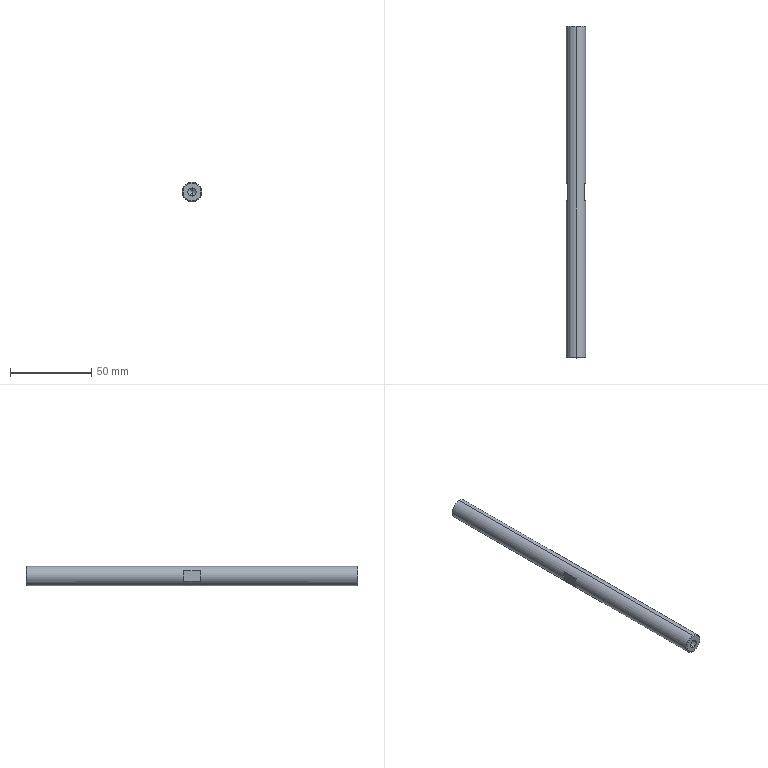Part | STEP file | 0-19-13 Support rod | 1 solid | 22 faces | box 12 x 204 x 12 mm | volume 22364 mm3 | cone 8 | plane 8 | cylinder 6 | commonest cylinder face diameters 5 x4 12 x2
STEP:
#1=CARTESIAN_POINT('',(0.,0.,0.));
#2=DIRECTION('',(0.,0.,1.));
#3=DIRECTION('',(1.,0.,0.));
#4=AXIS2_PLACEMENT_3D('',#1,#2,#3);
#5=CARTESIAN_POINT('',(0.,102.,5.5));
#6=VERTEX_POINT('',#5);
#7=CARTESIAN_POINT('',(0.,102.,-5.5));
#8=VERTEX_POINT('',#7);
#9=CARTESIAN_POINT('',(0.,102.,0.));
#10=DIRECTION('',(0.,1.,0.));
#11=DIRECTION('',(0.,0.,1.));
#12=AXIS2_PLACEMENT_3D('',#9,#10,#11);
#13=CIRCLE('',#12,5.5);
#14=CARTESIAN_POINT('',(0.,101.5,0.));
#15=DIRECTION('',(0.,-1.,0.));
#16=DIRECTION('',(0.,0.,-1.));
#17=AXIS2_PLACEMENT_3D('',#14,#15,#16);
#18=CONICAL_SURFACE('',#17,6.,0.7854);
#19=CARTESIAN_POINT('',(3.142,-0.5));
#20=DIRECTION('',(-1.,0.));
#21=VECTOR('',#20,1.);
#22=LINE('',#19,#21);
#23=(GEOMETRIC_REPRESENTATION_CONTEXT(2)PARAMETRIC_REPRESENTATION_CONTEXT()REPRESENTATION_CONTEXT('',''));
#24=DEFINITIONAL_REPRESENTATION('',(#22),#23);
#25=PCURVE('',#18,#24);
#26=CARTESIAN_POINT('',(6.,102.,0.));
#27=DIRECTION('',(0.,1.,0.));
#28=DIRECTION('',(0.,0.,1.));
#29=AXIS2_PLACEMENT_3D('',#26,#27,#28);
#30=PLANE('',#29);
#31=CARTESIAN_POINT('',(0.,-6.));
#32=DIRECTION('',(1.,0.));
#33=AXIS2_PLACEMENT_2D('',#31,#32);
#34=CIRCLE('',#33,5.5);
#35=(GEOMETRIC_REPRESENTATION_CONTEXT(2)PARAMETRIC_REPRESENTATION_CONTEXT()REPRESENTATION_CONTEXT('',''));
#36=DEFINITIONAL_REPRESENTATION('',(#34),#35);
#37=PCURVE('',#30,#36);
#38=SURFACE_CURVE('',#13,(#25,#37),.PCURVE_S1.);
#39=EDGE_CURVE('',#6,#8,#38,.T.);
#40=ORIENTED_EDGE('',*,*,#39,.F.);
#41=CARTESIAN_POINT('',(0.,101.5,6.));
#42=VERTEX_POINT('',#41);
#43=CARTESIAN_POINT('',(0.,101.5,6.));
#44=DIRECTION('',(0.,-0.7071,0.7071));
#45=VECTOR('',#44,1.);
#46=LINE('',#43,#45);
#47=CARTESIAN_POINT('',(3.142,0.));
#48=DIRECTION('',(0.,1.));
#49=VECTOR('',#48,1.);
#50=LINE('',#47,#49);
#51=(GEOMETRIC_REPRESENTATION_CONTEXT(2)PARAMETRIC_REPRESENTATION_CONTEXT()REPRESENTATION_CONTEXT('',''));
#52=DEFINITIONAL_REPRESENTATION('',(#50),#51);
#53=PCURVE('',#18,#52);
#54=CARTESIAN_POINT('',(0.,101.5,0.));
#55=DIRECTION('',(0.,-1.,0.));
#56=DIRECTION('',(0.,0.,-1.));
#57=AXIS2_PLACEMENT_3D('',#54,#55,#56);
#58=CONICAL_SURFACE('',#57,6.,0.7854);
#59=CARTESIAN_POINT('',(3.142,0.));
#60=DIRECTION('',(0.,1.));
#61=VECTOR('',#60,1.);
#62=LINE('',#59,#61);
#63=(GEOMETRIC_REPRESENTATION_CONTEXT(2)PARAMETRIC_REPRESENTATION_CONTEXT()REPRESENTATION_CONTEXT('',''));
#64=DEFINITIONAL_REPRESENTATION('',(#62),#63);
#65=PCURVE('',#58,#64);
#66=SURFACE_CURVE('',#46,(#53,#65),.PCURVE_S1.);
#67=EDGE_CURVE('',#6,#42,#66,.T.);
#68=ORIENTED_EDGE('',*,*,#67,.T.);
#69=CARTESIAN_POINT('',(0.,101.5,-6.));
#70=VERTEX_POINT('',#69);
#71=CARTESIAN_POINT('',(0.,101.5,0.));
#72=DIRECTION('',(0.,-1.,0.));
#73=DIRECTION('',(0.,0.,1.));
#74=AXIS2_PLACEMENT_3D('',#71,#72,#73);
#75=CIRCLE('',#74,6.);
#76=CARTESIAN_POINT('',(-3.142,0.));
#77=DIRECTION('',(1.,0.));
#78=VECTOR('',#77,1.);
#79=LINE('',#76,#78);
#80=(GEOMETRIC_REPRESENTATION_CONTEXT(2)PARAMETRIC_REPRESENTATION_CONTEXT()REPRESENTATION_CONTEXT('',''));
#81=DEFINITIONAL_REPRESENTATION('',(#79),#80);
#82=PCURVE('',#18,#81);
#83=CARTESIAN_POINT('',(0.,0.,0.));
#84=DIRECTION('',(0.,-1.,0.));
#85=DIRECTION('',(0.,0.,-1.));
#86=AXIS2_PLACEMENT_3D('',#83,#84,#85);
#87=CYLINDRICAL_SURFACE('',#86,6.);
#88=CARTESIAN_POINT('',(-3.142,-101.5));
#89=DIRECTION('',(1.,0.));
#90=VECTOR('',#89,1.);
#91=LINE('',#88,#90);
#92=(GEOMETRIC_REPRESENTATION_CONTEXT(2)PARAMETRIC_REPRESENTATION_CONTEXT()REPRESENTATION_CONTEXT('',''));
#93=DEFINITIONAL_REPRESENTATION('',(#91),#92);
#94=PCURVE('',#87,#93);
#95=SURFACE_CURVE('',#75,(#82,#94),.PCURVE_S1.);
#96=EDGE_CURVE('',#70,#42,#95,.T.);
#97=ORIENTED_EDGE('',*,*,#96,.F.);
#98=CARTESIAN_POINT('',(0.,101.5,-6.));
#99=DIRECTION('',(0.,-0.7071,-0.7071));
#100=VECTOR('',#99,1.);
#101=LINE('',#98,#100);
#102=CARTESIAN_POINT('',(0.,0.));
#103=DIRECTION('',(0.,1.));
#104=VECTOR('',#103,1.);
#105=LINE('',#102,#104);
#106=(GEOMETRIC_REPRESENTATION_CONTEXT(2)PARAMETRIC_REPRESENTATION_CONTEXT()REPRESENTATION_CONTEXT('',''));
#107=DEFINITIONAL_REPRESENTATION('',(#105),#106);
#108=PCURVE('',#18,#107);
#109=CARTESIAN_POINT('',(6.283,0.));
#110=DIRECTION('',(0.,1.));
#111=VECTOR('',#110,1.);
#112=LINE('',#109,#111);
#113=(GEOMETRIC_REPRESENTATION_CONTEXT(2)PARAMETRIC_REPRESENTATION_CONTEXT()REPRESENTATION_CONTEXT('',''));
#114=DEFINITIONAL_REPRESENTATION('',(#112),#113);
#115=PCURVE('',#58,#114);
#116=SURFACE_CURVE('',#101,(#108,#115),.PCURVE_S1.);
#117=EDGE_CURVE('',#8,#70,#116,.T.);
#118=ORIENTED_EDGE('',*,*,#117,.F.);
#119=EDGE_LOOP('',(#40,#68,#97,#118));
#120=FACE_BOUND('',#119,.T.);
#121=ADVANCED_FACE('',(#120),#18,.T.);
#122=CARTESIAN_POINT('',(0.,-102.,-5.5));
#123=VERTEX_POINT('',#122);
#124=CARTESIAN_POINT('',(0.,-102.,5.5));
#125=VERTEX_POINT('',#124);
#126=CARTESIAN_POINT('',(0.,-102.,0.));
#127=DIRECTION('',(0.,-1.,0.));
#128=DIRECTION('',(0.,0.,-1.));
#129=AXIS2_PLACEMENT_3D('',#126,#127,#128);
#130=CIRCLE('',#129,5.5);
#131=CARTESIAN_POINT('',(0.,-102.,0.));
#132=DIRECTION('',(0.,1.,0.));
#133=DIRECTION('',(0.,0.,1.));
#134=AXIS2_PLACEMENT_3D('',#131,#132,#133);
#135=CONICAL_SURFACE('',#134,5.5,0.7854);
#136=CARTESIAN_POINT('',(3.142,0.));
#137=DIRECTION('',(-1.,0.));
#138=VECTOR('',#137,1.);
#139=LINE('',#136,#138);
#140=(GEOMETRIC_REPRESENTATION_CONTEXT(2)PARAMETRIC_REPRESENTATION_CONTEXT()REPRESENTATION_CONTEXT('',''));
#141=DEFINITIONAL_REPRESENTATION('',(#139),#140);
#142=PCURVE('',#135,#141);
#143=CARTESIAN_POINT('',(6.,-102.,0.));
#144=DIRECTION('',(0.,-1.,0.));
#145=DIRECTION('',(0.,0.,-1.));
#146=AXIS2_PLACEMENT_3D('',#143,#144,#145);
#147=PLANE('',#146);
#148=CARTESIAN_POINT('',(0.,-6.));
#149=DIRECTION('',(1.,0.));
#150=AXIS2_PLACEMENT_2D('',#148,#149);
#151=CIRCLE('',#150,5.5);
#152=(GEOMETRIC_REPRESENTATION_CONTEXT(2)PARAMETRIC_REPRESENTATION_CONTEXT()REPRESENTATION_CONTEXT('',''));
#153=DEFINITIONAL_REPRESENTATION('',(#151),#152);
#154=PCURVE('',#147,#153);
#155=SURFACE_CURVE('',#130,(#142,#154),.PCURVE_S1.);
#156=EDGE_CURVE('',#123,#125,#155,.T.);
#157=ORIENTED_EDGE('',*,*,#156,.F.);
#158=CARTESIAN_POINT('',(0.,-101.5,-6.));
#159=VERTEX_POINT('',#158);
#160=CARTESIAN_POINT('',(0.,-102.,-5.5));
#161=DIRECTION('',(0.,0.7071,-0.7071));
#162=VECTOR('',#161,1.);
#163=LINE('',#160,#162);
#164=CARTESIAN_POINT('',(3.142,0.));
#165=DIRECTION('',(0.,1.));
#166=VECTOR('',#165,1.);
#167=LINE('',#164,#166);
#168=(GEOMETRIC_REPRESENTATION_CONTEXT(2)PARAMETRIC_REPRESENTATION_CONTEXT()REPRESENTATION_CONTEXT('',''));
#169=DEFINITIONAL_REPRESENTATION('',(#167),#168);
#170=PCURVE('',#135,#169);
#171=CARTESIAN_POINT('',(0.,-102.,0.));
#172=DIRECTION('',(0.,1.,0.));
#173=DIRECTION('',(0.,0.,1.));
#174=AXIS2_PLACEMENT_3D('',#171,#172,#173);
#175=CONICAL_SURFACE('',#174,5.5,0.7854);
#176=CARTESIAN_POINT('',(3.142,0.));
#177=DIRECTION('',(0.,1.));
#178=VECTOR('',#177,1.);
#179=LINE('',#176,#178);
#180=(GEOMETRIC_REPRESENTATION_CONTEXT(2)PARAMETRIC_REPRESENTATION_CONTEXT()REPRESENTATION_CONTEXT('',''));
#181=DEFINITIONAL_REPRESENTATION('',(#179),#180);
#182=PCURVE('',#175,#181);
#183=SURFACE_CURVE('',#163,(#170,#182),.PCURVE_S1.);
#184=EDGE_CURVE('',#123,#159,#183,.T.);
#185=ORIENTED_EDGE('',*,*,#184,.T.);
#186=CARTESIAN_POINT('',(0.,-101.5,6.));
#187=VERTEX_POINT('',#186);
#188=CARTESIAN_POINT('',(0.,-101.5,0.));
#189=DIRECTION('',(0.,1.,0.));
#190=DIRECTION('',(0.,0.,-1.));
#191=AXIS2_PLACEMENT_3D('',#188,#189,#190);
#192=CIRCLE('',#191,6.);
#193=CARTESIAN_POINT('',(-3.142,0.5));
#194=DIRECTION('',(1.,0.));
#195=VECTOR('',#194,1.);
#196=LINE('',#193,#195);
#197=(GEOMETRIC_REPRESENTATION_CONTEXT(2)PARAMETRIC_REPRESENTATION_CONTEXT()REPRESENTATION_CONTEXT('',''));
#198=DEFINITIONAL_REPRESENTATION('',(#196),#197);
#199=PCURVE('',#135,#198);
#200=CARTESIAN_POINT('',(6.283,101.5));
#201=DIRECTION('',(-1.,0.));
#202=VECTOR('',#201,1.);
#203=LINE('',#200,#202);
#204=(GEOMETRIC_REPRESENTATION_CONTEXT(2)PARAMETRIC_REPRESENTATION_CONTEXT()REPRESENTATION_CONTEXT('',''));
#205=DEFINITIONAL_REPRESENTATION('',(#203),#204);
#206=PCURVE('',#87,#205);
#207=SURFACE_CURVE('',#192,(#199,#206),.PCURVE_S1.);
#208=EDGE_CURVE('',#187,#159,#207,.T.);
#209=ORIENTED_EDGE('',*,*,#208,.F.);
#210=CARTESIAN_POINT('',(0.,-102.,5.5));
#211=DIRECTION('',(0.,0.7071,0.7071));
#212=VECTOR('',#211,1.);
#213=LINE('',#210,#212);
#214=CARTESIAN_POINT('',(0.,0.));
#215=DIRECTION('',(0.,1.));
#216=VECTOR('',#215,1.);
#217=LINE('',#214,#216);
#218=(GEOMETRIC_REPRESENTATION_CONTEXT(2)PARAMETRIC_REPRESENTATION_CONTEXT()REPRESENTATION_CONTEXT('',''));
#219=DEFINITIONAL_REPRESENTATION('',(#217),#218);
#220=PCURVE('',#135,#219);
#221=CARTESIAN_POINT('',(6.283,0.));
#222=DIRECTION('',(0.,1.));
#223=VECTOR('',#222,1.);
#224=LINE('',#221,#223);
#225=(GEOMETRIC_REPRESENTATION_CONTEXT(2)PARAMETRIC_REPRESENTATION_CONTEXT()REPRESENTATION_CONTEXT('',''));
#226=DEFINITIONAL_REPRESENTATION('',(#224),#225);
#227=PCURVE('',#175,#226);
#228=SURFACE_CURVE('',#213,(#220,#227),.PCURVE_S1.);
#229=EDGE_CURVE('',#125,#187,#228,.T.);
#230=ORIENTED_EDGE('',*,*,#229,.F.);
#231=EDGE_LOOP('',(#157,#185,#209,#230));
#232=FACE_BOUND('',#231,.T.);
#233=ADVANCED_FACE('',(#232),#135,.T.);
#234=CARTESIAN_POINT('',(0.,-87.,-2.5));
#235=VERTEX_POINT('',#234);
#236=CARTESIAN_POINT('',(0.,-102.,-2.5));
#237=VERTEX_POINT('',#236);
#238=CARTESIAN_POINT('',(0.,-102.,-2.5));
#239=DIRECTION('',(0.,-1.,0.));
#240=VECTOR('',#239,1.);
#241=LINE('',#238,#240);
#242=CARTESIAN_POINT('',(0.,-102.,0.));
#243=DIRECTION('',(0.,-1.,0.));
#244=DIRECTION('',(0.,0.,-1.));
#245=AXIS2_PLACEMENT_3D('',#242,#243,#244);
#246=CYLINDRICAL_SURFACE('',#245,2.5);
#247=CARTESIAN_POINT('',(6.283,0.));
#248=DIRECTION('',(0.,1.));
#249=VECTOR('',#248,1.);
#250=LINE('',#247,#249);
#251=(GEOMETRIC_REPRESENTATION_CONTEXT(2)PARAMETRIC_REPRESENTATION_CONTEXT()REPRESENTATION_CONTEXT('',''));
#252=DEFINITIONAL_REPRESENTATION('',(#250),#251);
#253=PCURVE('',#246,#252);
#254=CARTESIAN_POINT('',(0.,-102.,0.));
#255=DIRECTION('',(0.,-1.,0.));
#256=DIRECTION('',(0.,0.,-1.));
#257=AXIS2_PLACEMENT_3D('',#254,#255,#256);
#258=CYLINDRICAL_SURFACE('',#257,2.5);
#259=CARTESIAN_POINT('',(0.,0.));
#260=DIRECTION('',(0.,1.));
#261=VECTOR('',#260,1.);
#262=LINE('',#259,#261);
#263=(GEOMETRIC_REPRESENTATION_CONTEXT(2)PARAMETRIC_REPRESENTATION_CONTEXT()REPRESENTATION_CONTEXT('',''));
#264=DEFINITIONAL_REPRESENTATION('',(#262),#263);
#265=PCURVE('',#258,#264);
#266=SURFACE_CURVE('',#241,(#253,#265),.PCURVE_S1.);
#267=EDGE_CURVE('',#235,#237,#266,.T.);
#268=ORIENTED_EDGE('',*,*,#267,.T.);
#269=CARTESIAN_POINT('',(0.,-102.,2.5));
#270=VERTEX_POINT('',#269);
#271=CARTESIAN_POINT('',(0.,-102.,0.));
#272=DIRECTION('',(0.,-1.,0.));
#273=DIRECTION('',(0.,0.,-1.));
#274=AXIS2_PLACEMENT_3D('',#271,#272,#273);
#275=CIRCLE('',#274,2.5);
#276=CARTESIAN_POINT('',(0.,0.));
#277=DIRECTION('',(1.,0.));
#278=VECTOR('',#277,1.);
#279=LINE('',#276,#278);
#280=(GEOMETRIC_REPRESENTATION_CONTEXT(2)PARAMETRIC_REPRESENTATION_CONTEXT()REPRESENTATION_CONTEXT('',''));
#281=DEFINITIONAL_REPRESENTATION('',(#279),#280);
#282=PCURVE('',#246,#281);
#283=CARTESIAN_POINT('',(0.,-6.));
#284=DIRECTION('',(1.,0.));
#285=AXIS2_PLACEMENT_2D('',#283,#284);
#286=CIRCLE('',#285,2.5);
#287=(GEOMETRIC_REPRESENTATION_CONTEXT(2)PARAMETRIC_REPRESENTATION_CONTEXT()REPRESENTATION_CONTEXT('',''));
#288=DEFINITIONAL_REPRESENTATION('',(#286),#287);
#289=PCURVE('',#147,#288);
#290=SURFACE_CURVE('',#275,(#282,#289),.PCURVE_S1.);
#291=EDGE_CURVE('',#270,#237,#290,.T.);
#292=ORIENTED_EDGE('',*,*,#291,.F.);
#293=CARTESIAN_POINT('',(0.,-87.,2.5));
#294=VERTEX_POINT('',#293);
#295=CARTESIAN_POINT('',(0.,-102.,2.5));
#296=DIRECTION('',(0.,-1.,0.));
#297=VECTOR('',#296,1.);
#298=LINE('',#295,#297);
#299=CARTESIAN_POINT('',(3.142,0.));
#300=DIRECTION('',(0.,1.));
#301=VECTOR('',#300,1.);
#302=LINE('',#299,#301);
#303=(GEOMETRIC_REPRESENTATION_CONTEXT(2)PARAMETRIC_REPRESENTATION_CONTEXT()REPRESENTATION_CONTEXT('',''));
#304=DEFINITIONAL_REPRESENTATION('',(#302),#303);
#305=PCURVE('',#246,#304);
#306=CARTESIAN_POINT('',(3.142,0.));
#307=DIRECTION('',(0.,1.));
#308=VECTOR('',#307,1.);
#309=LINE('',#306,#308);
#310=(GEOMETRIC_REPRESENTATION_CONTEXT(2)PARAMETRIC_REPRESENTATION_CONTEXT()REPRESENTATION_CONTEXT('',''));
#311=DEFINITIONAL_REPRESENTATION('',(#309),#310);
#312=PCURVE('',#258,#311);
#313=SURFACE_CURVE('',#298,(#305,#312),.PCURVE_S1.);
#314=EDGE_CURVE('',#294,#270,#313,.T.);
#315=ORIENTED_EDGE('',*,*,#314,.F.);
#316=CARTESIAN_POINT('',(0.,-87.,0.));
#317=DIRECTION('',(0.,-1.,0.));
#318=DIRECTION('',(0.,0.,-1.));
#319=AXIS2_PLACEMENT_3D('',#316,#317,#318);
#320=CIRCLE('',#319,2.5);
#321=CARTESIAN_POINT('',(0.,-15.));
#322=DIRECTION('',(1.,0.));
#323=VECTOR('',#322,1.);
#324=LINE('',#321,#323);
#325=(GEOMETRIC_REPRESENTATION_CONTEXT(2)PARAMETRIC_REPRESENTATION_CONTEXT()REPRESENTATION_CONTEXT('',''));
#326=DEFINITIONAL_REPRESENTATION('',(#324),#325);
#327=PCURVE('',#246,#326);
#328=CARTESIAN_POINT('',(0.,-87.,0.));
#329=DIRECTION('',(0.,-1.,0.));
#330=DIRECTION('',(0.,0.,-1.));
#331=AXIS2_PLACEMENT_3D('',#328,#329,#330);
#332=CONICAL_SURFACE('',#331,2.5,1.03);
#333=CARTESIAN_POINT('',(0.,0.));
#334=DIRECTION('',(1.,0.));
#335=VECTOR('',#334,1.);
#336=LINE('',#333,#335);
#337=(GEOMETRIC_REPRESENTATION_CONTEXT(2)PARAMETRIC_REPRESENTATION_CONTEXT()REPRESENTATION_CONTEXT('',''));
#338=DEFINITIONAL_REPRESENTATION('',(#336),#337);
#339=PCURVE('',#332,#338);
#340=SURFACE_CURVE('',#320,(#327,#339),.PCURVE_S1.);
#341=EDGE_CURVE('',#294,#235,#340,.T.);
#342=ORIENTED_EDGE('',*,*,#341,.T.);
#343=EDGE_LOOP('',(#268,#292,#315,#342));
#344=FACE_BOUND('',#343,.F.);
#345=ADVANCED_FACE('',(#344),#246,.F.);
#346=ORIENTED_EDGE('',*,*,#341,.F.);
#347=CARTESIAN_POINT('',(0.,-85.498,0.));
#348=VERTEX_POINT('',#347);
#349=CARTESIAN_POINT('',(0.,-87.,2.5));
#350=DIRECTION('',(0.,-0.515,0.8572));
#351=VECTOR('',#350,1.);
#352=LINE('',#349,#351);
#353=CARTESIAN_POINT('',(3.142,0.));
#354=DIRECTION('',(0.,1.));
#355=VECTOR('',#354,1.);
#356=LINE('',#353,#355);
#357=(GEOMETRIC_REPRESENTATION_CONTEXT(2)PARAMETRIC_REPRESENTATION_CONTEXT()REPRESENTATION_CONTEXT('',''));
#358=DEFINITIONAL_REPRESENTATION('',(#356),#357);
#359=PCURVE('',#332,#358);
#360=CARTESIAN_POINT('',(0.,-87.,0.));
#361=DIRECTION('',(0.,-1.,0.));
#362=DIRECTION('',(0.,0.,-1.));
#363=AXIS2_PLACEMENT_3D('',#360,#361,#362);
#364=CONICAL_SURFACE('',#363,2.5,1.03);
#365=CARTESIAN_POINT('',(3.142,0.));
#366=DIRECTION('',(0.,1.));
#367=VECTOR('',#366,1.);
#368=LINE('',#365,#367);
#369=(GEOMETRIC_REPRESENTATION_CONTEXT(2)PARAMETRIC_REPRESENTATION_CONTEXT()REPRESENTATION_CONTEXT('',''));
#370=DEFINITIONAL_REPRESENTATION('',(#368),#369);
#371=PCURVE('',#364,#370);
#372=SURFACE_CURVE('',#352,(#359,#371),.PCURVE_S1.);
#373=EDGE_CURVE('',#348,#294,#372,.T.);
#374=ORIENTED_EDGE('',*,*,#373,.F.);
#375=CARTESIAN_POINT('',(0.,-87.,-2.5));
#376=DIRECTION('',(0.,-0.515,-0.8572));
#377=VECTOR('',#376,1.);
#378=LINE('',#375,#377);
#379=CARTESIAN_POINT('',(6.283,0.));
#380=DIRECTION('',(0.,1.));
#381=VECTOR('',#380,1.);
#382=LINE('',#379,#381);
#383=(GEOMETRIC_REPRESENTATION_CONTEXT(2)PARAMETRIC_REPRESENTATION_CONTEXT()REPRESENTATION_CONTEXT('',''));
#384=DEFINITIONAL_REPRESENTATION('',(#382),#383);
#385=PCURVE('',#332,#384);
#386=CARTESIAN_POINT('',(0.,0.));
#387=DIRECTION('',(0.,1.));
#388=VECTOR('',#387,1.);
#389=LINE('',#386,#388);
#390=(GEOMETRIC_REPRESENTATION_CONTEXT(2)PARAMETRIC_REPRESENTATION_CONTEXT()REPRESENTATION_CONTEXT('',''));
#391=DEFINITIONAL_REPRESENTATION('',(#389),#390);
#392=PCURVE('',#364,#391);
#393=SURFACE_CURVE('',#378,(#385,#392),.PCURVE_S1.);
#394=EDGE_CURVE('',#348,#235,#393,.T.);
#395=ORIENTED_EDGE('',*,*,#394,.T.);
#396=EDGE_LOOP('',(#346,#374,#395));
#397=FACE_BOUND('',#396,.F.);
#398=ADVANCED_FACE('',(#397),#332,.F.);
#399=CARTESIAN_POINT('',(0.,87.,2.5));
#400=VERTEX_POINT('',#399);
#401=CARTESIAN_POINT('',(0.,102.,2.5));
#402=VERTEX_POINT('',#401);
#403=CARTESIAN_POINT('',(0.,102.,2.5));
#404=DIRECTION('',(0.,1.,0.));
#405=VECTOR('',#404,1.);
#406=LINE('',#403,#405);
#407=CARTESIAN_POINT('',(0.,102.,0.));
#408=DIRECTION('',(0.,1.,0.));
#409=DIRECTION('',(0.,0.,1.));
#410=AXIS2_PLACEMENT_3D('',#407,#408,#409);
#411=CYLINDRICAL_SURFACE('',#410,2.5);
#412=CARTESIAN_POINT('',(6.283,0.));
#413=DIRECTION('',(0.,1.));
#414=VECTOR('',#413,1.);
#415=LINE('',#412,#414);
#416=(GEOMETRIC_REPRESENTATION_CONTEXT(2)PARAMETRIC_REPRESENTATION_CONTEXT()REPRESENTATION_CONTEXT('',''));
#417=DEFINITIONAL_REPRESENTATION('',(#415),#416);
#418=PCURVE('',#411,#417);
#419=CARTESIAN_POINT('',(0.,102.,0.));
#420=DIRECTION('',(0.,1.,0.));
#421=DIRECTION('',(0.,0.,1.));
#422=AXIS2_PLACEMENT_3D('',#419,#420,#421);
#423=CYLINDRICAL_SURFACE('',#422,2.5);
#424=CARTESIAN_POINT('',(0.,0.));
#425=DIRECTION('',(0.,1.));
#426=VECTOR('',#425,1.);
#427=LINE('',#424,#426);
#428=(GEOMETRIC_REPRESENTATION_CONTEXT(2)PARAMETRIC_REPRESENTATION_CONTEXT()REPRESENTATION_CONTEXT('',''));
#429=DEFINITIONAL_REPRESENTATION('',(#427),#428);
#430=PCURVE('',#423,#429);
#431=SURFACE_CURVE('',#406,(#418,#430),.PCURVE_S1.);
#432=EDGE_CURVE('',#400,#402,#431,.T.);
#433=ORIENTED_EDGE('',*,*,#432,.T.);
#434=CARTESIAN_POINT('',(0.,102.,-2.5));
#435=VERTEX_POINT('',#434);
#436=CARTESIAN_POINT('',(0.,102.,0.));
#437=DIRECTION('',(0.,1.,0.));
#438=DIRECTION('',(0.,0.,1.));
#439=AXIS2_PLACEMENT_3D('',#436,#437,#438);
#440=CIRCLE('',#439,2.5);
#441=CARTESIAN_POINT('',(0.,0.));
#442=DIRECTION('',(1.,0.));
#443=VECTOR('',#442,1.);
#444=LINE('',#441,#443);
#445=(GEOMETRIC_REPRESENTATION_CONTEXT(2)PARAMETRIC_REPRESENTATION_CONTEXT()REPRESENTATION_CONTEXT('',''));
#446=DEFINITIONAL_REPRESENTATION('',(#444),#445);
#447=PCURVE('',#411,#446);
#448=CARTESIAN_POINT('',(0.,-6.));
#449=DIRECTION('',(1.,0.));
#450=AXIS2_PLACEMENT_2D('',#448,#449);
#451=CIRCLE('',#450,2.5);
#452=(GEOMETRIC_REPRESENTATION_CONTEXT(2)PARAMETRIC_REPRESENTATION_CONTEXT()REPRESENTATION_CONTEXT('',''));
#453=DEFINITIONAL_REPRESENTATION('',(#451),#452);
#454=PCURVE('',#30,#453);
#455=SURFACE_CURVE('',#440,(#447,#454),.PCURVE_S1.);
#456=EDGE_CURVE('',#435,#402,#455,.T.);
#457=ORIENTED_EDGE('',*,*,#456,.F.);
#458=CARTESIAN_POINT('',(0.,87.,-2.5));
#459=VERTEX_POINT('',#458);
#460=CARTESIAN_POINT('',(0.,102.,-2.5));
#461=DIRECTION('',(0.,1.,0.));
#462=VECTOR('',#461,1.);
#463=LINE('',#460,#462);
#464=CARTESIAN_POINT('',(3.142,0.));
#465=DIRECTION('',(0.,1.));
#466=VECTOR('',#465,1.);
#467=LINE('',#464,#466);
#468=(GEOMETRIC_REPRESENTATION_CONTEXT(2)PARAMETRIC_REPRESENTATION_CONTEXT()REPRESENTATION_CONTEXT('',''));
#469=DEFINITIONAL_REPRESENTATION('',(#467),#468);
#470=PCURVE('',#411,#469);
#471=CARTESIAN_POINT('',(3.142,0.));
#472=DIRECTION('',(0.,1.));
#473=VECTOR('',#472,1.);
#474=LINE('',#471,#473);
#475=(GEOMETRIC_REPRESENTATION_CONTEXT(2)PARAMETRIC_REPRESENTATION_CONTEXT()REPRESENTATION_CONTEXT('',''));
#476=DEFINITIONAL_REPRESENTATION('',(#474),#475);
#477=PCURVE('',#423,#476);
#478=SURFACE_CURVE('',#463,(#470,#477),.PCURVE_S1.);
#479=EDGE_CURVE('',#459,#435,#478,.T.);
#480=ORIENTED_EDGE('',*,*,#479,.F.);
#481=CARTESIAN_POINT('',(0.,87.,0.));
#482=DIRECTION('',(0.,1.,0.));
#483=DIRECTION('',(0.,0.,1.));
#484=AXIS2_PLACEMENT_3D('',#481,#482,#483);
#485=CIRCLE('',#484,2.5);
#486=CARTESIAN_POINT('',(0.,-15.));
#487=DIRECTION('',(1.,0.));
#488=VECTOR('',#487,1.);
#489=LINE('',#486,#488);
#490=(GEOMETRIC_REPRESENTATION_CONTEXT(2)PARAMETRIC_REPRESENTATION_CONTEXT()REPRESENTATION_CONTEXT('',''));
#491=DEFINITIONAL_REPRESENTATION('',(#489),#490);
#492=PCURVE('',#411,#491);
#493=CARTESIAN_POINT('',(0.,87.,0.));
#494=DIRECTION('',(0.,1.,0.));
#495=DIRECTION('',(0.,0.,1.));
#496=AXIS2_PLACEMENT_3D('',#493,#494,#495);
#497=CONICAL_SURFACE('',#496,2.5,1.03);
#498=CARTESIAN_POINT('',(0.,0.));
#499=DIRECTION('',(1.,0.));
#500=VECTOR('',#499,1.);
#501=LINE('',#498,#500);
#502=(GEOMETRIC_REPRESENTATION_CONTEXT(2)PARAMETRIC_REPRESENTATION_CONTEXT()REPRESENTATION_CONTEXT('',''));
#503=DEFINITIONAL_REPRESENTATION('',(#501),#502);
#504=PCURVE('',#497,#503);
#505=SURFACE_CURVE('',#485,(#492,#504),.PCURVE_S1.);
#506=EDGE_CURVE('',#459,#400,#505,.T.);
#507=ORIENTED_EDGE('',*,*,#506,.T.);
#508=EDGE_LOOP('',(#433,#457,#480,#507));
#509=FACE_BOUND('',#508,.F.);
#510=ADVANCED_FACE('',(#509),#411,.F.);
#511=ORIENTED_EDGE('',*,*,#506,.F.);
#512=CARTESIAN_POINT('',(0.,85.498,0.));
#513=VERTEX_POINT('',#512);
#514=CARTESIAN_POINT('',(0.,87.,-2.5));
#515=DIRECTION('',(0.,0.515,-0.8572));
#516=VECTOR('',#515,1.);
#517=LINE('',#514,#516);
#518=CARTESIAN_POINT('',(3.142,0.));
#519=DIRECTION('',(0.,1.));
#520=VECTOR('',#519,1.);
#521=LINE('',#518,#520);
#522=(GEOMETRIC_REPRESENTATION_CONTEXT(2)PARAMETRIC_REPRESENTATION_CONTEXT()REPRESENTATION_CONTEXT('',''));
#523=DEFINITIONAL_REPRESENTATION('',(#521),#522);
#524=PCURVE('',#497,#523);
#525=CARTESIAN_POINT('',(0.,87.,0.));
#526=DIRECTION('',(0.,1.,0.));
#527=DIRECTION('',(0.,0.,1.));
#528=AXIS2_PLACEMENT_3D('',#525,#526,#527);
#529=CONICAL_SURFACE('',#528,2.5,1.03);
#530=CARTESIAN_POINT('',(3.142,0.));
#531=DIRECTION('',(0.,1.));
#532=VECTOR('',#531,1.);
#533=LINE('',#530,#532);
#534=(GEOMETRIC_REPRESENTATION_CONTEXT(2)PARAMETRIC_REPRESENTATION_CONTEXT()REPRESENTATION_CONTEXT('',''));
#535=DEFINITIONAL_REPRESENTATION('',(#533),#534);
#536=PCURVE('',#529,#535);
#537=SURFACE_CURVE('',#517,(#524,#536),.PCURVE_S1.);
#538=EDGE_CURVE('',#513,#459,#537,.T.);
#539=ORIENTED_EDGE('',*,*,#538,.F.);
#540=CARTESIAN_POINT('',(0.,87.,2.5));
#541=DIRECTION('',(0.,0.515,0.8572));
#542=VECTOR('',#541,1.);
#543=LINE('',#540,#542);
#544=CARTESIAN_POINT('',(6.283,0.));
#545=DIRECTION('',(0.,1.));
#546=VECTOR('',#545,1.);
#547=LINE('',#544,#546);
#548=(GEOMETRIC_REPRESENTATION_CONTEXT(2)PARAMETRIC_REPRESENTATION_CONTEXT()REPRESENTATION_CONTEXT('',''));
#549=DEFINITIONAL_REPRESENTATION('',(#547),#548);
#550=PCURVE('',#497,#549);
#551=CARTESIAN_POINT('',(0.,0.));
#552=DIRECTION('',(0.,1.));
#553=VECTOR('',#552,1.);
#554=LINE('',#551,#553);
#555=(GEOMETRIC_REPRESENTATION_CONTEXT(2)PARAMETRIC_REPRESENTATION_CONTEXT()REPRESENTATION_CONTEXT('',''));
#556=DEFINITIONAL_REPRESENTATION('',(#554),#555);
#557=PCURVE('',#529,#556);
#558=SURFACE_CURVE('',#543,(#550,#557),.PCURVE_S1.);
#559=EDGE_CURVE('',#513,#400,#558,.T.);
#560=ORIENTED_EDGE('',*,*,#559,.T.);
#561=EDGE_LOOP('',(#511,#539,#560));
#562=FACE_BOUND('',#561,.F.);
#563=ADVANCED_FACE('',(#562),#497,.F.);
#564=CARTESIAN_POINT('',(5.,-5.,3.317));
#565=VERTEX_POINT('',#564);
#566=CARTESIAN_POINT('',(5.,-5.,-3.317));
#567=VERTEX_POINT('',#566);
#568=CARTESIAN_POINT('',(0.,-5.,0.));
#569=DIRECTION('',(0.,1.,0.));
#570=DIRECTION('',(0.,0.,-1.));
#571=AXIS2_PLACEMENT_3D('',#568,#569,#570);
#572=CIRCLE('',#571,6.);
#573=CARTESIAN_POINT('',(6.283,5.));
#574=DIRECTION('',(-1.,0.));
#575=VECTOR('',#574,1.);
#576=LINE('',#573,#575);
#577=(GEOMETRIC_REPRESENTATION_CONTEXT(2)PARAMETRIC_REPRESENTATION_CONTEXT()REPRESENTATION_CONTEXT('',''));
#578=DEFINITIONAL_REPRESENTATION('',(#576),#577);
#579=PCURVE('',#87,#578);
#580=CARTESIAN_POINT('',(0.,-5.,0.));
#581=DIRECTION('',(0.,-1.,0.));
#582=DIRECTION('',(0.,0.,-1.));
#583=AXIS2_PLACEMENT_3D('',#580,#581,#582);
#584=PLANE('',#583);
#585=CARTESIAN_POINT('',(6.,0.));
#586=CARTESIAN_POINT('',(6.,-10.392));
#587=CARTESIAN_POINT('',(-3.,-5.196));
#588=CARTESIAN_POINT('',(-12.,0.));
#589=CARTESIAN_POINT('',(-3.,5.196));
#590=CARTESIAN_POINT('',(6.,10.392));
#591=CARTESIAN_POINT('',(6.,0.));
#592=(BOUNDED_CURVE()B_SPLINE_CURVE(2,(#585,#586,#587,#588,#589,#590,#591),.UNSPECIFIED.,.T.,.F.)B_SPLINE_CURVE_WITH_KNOTS((1,2,2,2,2,1),(-2.094,0.,2.094,4.189,6.283,8.378),.UNSPECIFIED.)CURVE()GEOMETRIC_REPRESENTATION_ITEM()RATIONAL_B_SPLINE_CURVE((1.,0.5,1.,0.5,1.,0.5,1.))REPRESENTATION_ITEM(''));
#593=(GEOMETRIC_REPRESENTATION_CONTEXT(2)PARAMETRIC_REPRESENTATION_CONTEXT()REPRESENTATION_CONTEXT('',''));
#594=DEFINITIONAL_REPRESENTATION('',(#592),#593);
#595=PCURVE('',#584,#594);
#596=SURFACE_CURVE('',#572,(#579,#595),.PCURVE_S1.);
#597=EDGE_CURVE('',#565,#567,#596,.T.);
#598=ORIENTED_EDGE('',*,*,#597,.F.);
#599=CARTESIAN_POINT('',(5.,5.,3.317));
#600=VERTEX_POINT('',#599);
#601=CARTESIAN_POINT('',(5.,-5.,3.317));
#602=DIRECTION('',(0.,1.,0.));
#603=VECTOR('',#602,1.);
#604=LINE('',#601,#603);
#605=CARTESIAN_POINT('',(2.156,5.));
#606=DIRECTION('',(0.,-1.));
#607=VECTOR('',#606,1.);
#608=LINE('',#605,#607);
#609=(GEOMETRIC_REPRESENTATION_CONTEXT(2)PARAMETRIC_REPRESENTATION_CONTEXT()REPRESENTATION_CONTEXT('',''));
#610=DEFINITIONAL_REPRESENTATION('',(#608),#609);
#611=PCURVE('',#87,#610);
#612=CARTESIAN_POINT('',(5.,-5.,3.317));
#613=DIRECTION('',(-1.,0.,0.));
#614=DIRECTION('',(0.,0.,1.));
#615=AXIS2_PLACEMENT_3D('',#612,#613,#614);
#616=PLANE('',#615);
#617=CARTESIAN_POINT('',(0.,0.));
#618=DIRECTION('',(0.,1.));
#619=VECTOR('',#618,1.);
#620=LINE('',#617,#619);
#621=(GEOMETRIC_REPRESENTATION_CONTEXT(2)PARAMETRIC_REPRESENTATION_CONTEXT()REPRESENTATION_CONTEXT('',''));
#622=DEFINITIONAL_REPRESENTATION('',(#620),#621);
#623=PCURVE('',#616,#622);
#624=SURFACE_CURVE('',#604,(#611,#623),.PCURVE_S1.);
#625=EDGE_CURVE('',#565,#600,#624,.T.);
#626=ORIENTED_EDGE('',*,*,#625,.T.);
#627=CARTESIAN_POINT('',(5.,5.,-3.317));
#628=VERTEX_POINT('',#627);
#629=CARTESIAN_POINT('',(0.,5.,0.));
#630=DIRECTION('',(0.,1.,0.));
#631=DIRECTION('',(0.,0.,-1.));
#632=AXIS2_PLACEMENT_3D('',#629,#630,#631);
#633=CIRCLE('',#632,6.);
#634=CARTESIAN_POINT('',(6.283,-5.));
#635=DIRECTION('',(-1.,0.));
#636=VECTOR('',#635,1.);
#637=LINE('',#634,#636);
#638=(GEOMETRIC_REPRESENTATION_CONTEXT(2)PARAMETRIC_REPRESENTATION_CONTEXT()REPRESENTATION_CONTEXT('',''));
#639=DEFINITIONAL_REPRESENTATION('',(#637),#638);
#640=PCURVE('',#87,#639);
#641=CARTESIAN_POINT('',(0.,5.,0.));
#642=DIRECTION('',(0.,-1.,0.));
#643=DIRECTION('',(0.,0.,-1.));
#644=AXIS2_PLACEMENT_3D('',#641,#642,#643);
#645=PLANE('',#644);
#646=CARTESIAN_POINT('',(6.,0.));
#647=CARTESIAN_POINT('',(6.,-10.392));
#648=CARTESIAN_POINT('',(-3.,-5.196));
#649=CARTESIAN_POINT('',(-12.,0.));
#650=CARTESIAN_POINT('',(-3.,5.196));
#651=CARTESIAN_POINT('',(6.,10.392));
#652=CARTESIAN_POINT('',(6.,0.));
#653=(BOUNDED_CURVE()B_SPLINE_CURVE(2,(#646,#647,#648,#649,#650,#651,#652),.UNSPECIFIED.,.T.,.F.)B_SPLINE_CURVE_WITH_KNOTS((1,2,2,2,2,1),(-2.094,0.,2.094,4.189,6.283,8.378),.UNSPECIFIED.)CURVE()GEOMETRIC_REPRESENTATION_ITEM()RATIONAL_B_SPLINE_CURVE((1.,0.5,1.,0.5,1.,0.5,1.))REPRESENTATION_ITEM(''));
#654=(GEOMETRIC_REPRESENTATION_CONTEXT(2)PARAMETRIC_REPRESENTATION_CONTEXT()REPRESENTATION_CONTEXT('',''));
#655=DEFINITIONAL_REPRESENTATION('',(#653),#654);
#656=PCURVE('',#645,#655);
#657=SURFACE_CURVE('',#633,(#640,#656),.PCURVE_S1.);
#658=EDGE_CURVE('',#600,#628,#657,.T.);
#659=ORIENTED_EDGE('',*,*,#658,.T.);
#660=CARTESIAN_POINT('',(5.,-5.,-3.317));
#661=DIRECTION('',(0.,1.,0.));
#662=VECTOR('',#661,1.);
#663=LINE('',#660,#662);
#664=CARTESIAN_POINT('',(0.9851,5.));
#665=DIRECTION('',(0.,-1.));
#666=VECTOR('',#665,1.);
#667=LINE('',#664,#666);
#668=(GEOMETRIC_REPRESENTATION_CONTEXT(2)PARAMETRIC_REPRESENTATION_CONTEXT()REPRESENTATION_CONTEXT('',''));
#669=DEFINITIONAL_REPRESENTATION('',(#667),#668);
#670=PCURVE('',#87,#669);
#671=CARTESIAN_POINT('',(-6.633,0.));
#672=DIRECTION('',(0.,1.));
#673=VECTOR('',#672,1.);
#674=LINE('',#671,#673);
#675=(GEOMETRIC_REPRESENTATION_CONTEXT(2)PARAMETRIC_REPRESENTATION_CONTEXT()REPRESENTATION_CONTEXT('',''));
#676=DEFINITIONAL_REPRESENTATION('',(#674),#675);
#677=PCURVE('',#616,#676);
#678=SURFACE_CURVE('',#663,(#670,#677),.PCURVE_S1.);
#679=EDGE_CURVE('',#567,#628,#678,.T.);
#680=ORIENTED_EDGE('',*,*,#679,.F.);
#681=EDGE_LOOP('',(#598,#626,#659,#680));
#682=FACE_BOUND('',#681,.T.);
#683=ORIENTED_EDGE('',*,*,#96,.T.);
#684=CARTESIAN_POINT('',(0.,0.,6.));
#685=DIRECTION('',(0.,-1.,0.));
#686=VECTOR('',#685,1.);
#687=LINE('',#684,#686);
#688=CARTESIAN_POINT('',(3.142,0.));
#689=DIRECTION('',(0.,1.));
#690=VECTOR('',#689,1.);
#691=LINE('',#688,#690);
#692=(GEOMETRIC_REPRESENTATION_CONTEXT(2)PARAMETRIC_REPRESENTATION_CONTEXT()REPRESENTATION_CONTEXT('',''));
#693=DEFINITIONAL_REPRESENTATION('',(#691),#692);
#694=PCURVE('',#87,#693);
#695=CARTESIAN_POINT('',(0.,0.,0.));
#696=DIRECTION('',(0.,-1.,0.));
#697=DIRECTION('',(0.,0.,-1.));
#698=AXIS2_PLACEMENT_3D('',#695,#696,#697);
#699=CYLINDRICAL_SURFACE('',#698,6.);
#700=CARTESIAN_POINT('',(3.142,0.));
#701=DIRECTION('',(0.,1.));
#702=VECTOR('',#701,1.);
#703=LINE('',#700,#702);
#704=(GEOMETRIC_REPRESENTATION_CONTEXT(2)PARAMETRIC_REPRESENTATION_CONTEXT()REPRESENTATION_CONTEXT('',''));
#705=DEFINITIONAL_REPRESENTATION('',(#703),#704);
#706=PCURVE('',#699,#705);
#707=SURFACE_CURVE('',#687,(#694,#706),.PCURVE_S1.);
#708=EDGE_CURVE('',#42,#187,#707,.T.);
#709=ORIENTED_EDGE('',*,*,#708,.T.);
#710=ORIENTED_EDGE('',*,*,#208,.T.);
#711=CARTESIAN_POINT('',(0.,0.,-6.));
#712=DIRECTION('',(0.,-1.,0.));
#713=VECTOR('',#712,1.);
#714=LINE('',#711,#713);
#715=CARTESIAN_POINT('',(0.,0.));
#716=DIRECTION('',(0.,1.));
#717=VECTOR('',#716,1.);
#718=LINE('',#715,#717);
#719=(GEOMETRIC_REPRESENTATION_CONTEXT(2)PARAMETRIC_REPRESENTATION_CONTEXT()REPRESENTATION_CONTEXT('',''));
#720=DEFINITIONAL_REPRESENTATION('',(#718),#719);
#721=PCURVE('',#87,#720);
#722=CARTESIAN_POINT('',(6.283,0.));
#723=DIRECTION('',(0.,1.));
#724=VECTOR('',#723,1.);
#725=LINE('',#722,#724);
#726=(GEOMETRIC_REPRESENTATION_CONTEXT(2)PARAMETRIC_REPRESENTATION_CONTEXT()REPRESENTATION_CONTEXT('',''));
#727=DEFINITIONAL_REPRESENTATION('',(#725),#726);
#728=PCURVE('',#699,#727);
#729=SURFACE_CURVE('',#714,(#721,#728),.PCURVE_S1.);
#730=EDGE_CURVE('',#70,#159,#729,.T.);
#731=ORIENTED_EDGE('',*,*,#730,.F.);
#732=EDGE_LOOP('',(#683,#709,#710,#731));
#733=FACE_BOUND('',#732,.T.);
#734=ADVANCED_FACE('',(#682,#733),#87,.T.);
#735=ORIENTED_EDGE('',*,*,#708,.F.);
#736=CARTESIAN_POINT('',(0.,101.5,0.));
#737=DIRECTION('',(0.,-1.,0.));
#738=DIRECTION('',(0.,0.,1.));
#739=AXIS2_PLACEMENT_3D('',#736,#737,#738);
#740=CIRCLE('',#739,6.);
#741=CARTESIAN_POINT('',(3.142,-101.5));
#742=DIRECTION('',(1.,0.));
#743=VECTOR('',#742,1.);
#744=LINE('',#741,#743);
#745=(GEOMETRIC_REPRESENTATION_CONTEXT(2)PARAMETRIC_REPRESENTATION_CONTEXT()REPRESENTATION_CONTEXT('',''));
#746=DEFINITIONAL_REPRESENTATION('',(#744),#745);
#747=PCURVE('',#699,#746);
#748=CARTESIAN_POINT('',(3.142,0.));
#749=DIRECTION('',(1.,0.));
#750=VECTOR('',#749,1.);
#751=LINE('',#748,#750);
#752=(GEOMETRIC_REPRESENTATION_CONTEXT(2)PARAMETRIC_REPRESENTATION_CONTEXT()REPRESENTATION_CONTEXT('',''));
#753=DEFINITIONAL_REPRESENTATION('',(#751),#752);
#754=PCURVE('',#58,#753);
#755=SURFACE_CURVE('',#740,(#747,#754),.PCURVE_S1.);
#756=EDGE_CURVE('',#42,#70,#755,.T.);
#757=ORIENTED_EDGE('',*,*,#756,.T.);
#758=ORIENTED_EDGE('',*,*,#730,.T.);
#759=CARTESIAN_POINT('',(0.,-101.5,0.));
#760=DIRECTION('',(0.,1.,0.));
#761=DIRECTION('',(0.,0.,-1.));
#762=AXIS2_PLACEMENT_3D('',#759,#760,#761);
#763=CIRCLE('',#762,6.);
#764=CARTESIAN_POINT('',(6.283,101.5));
#765=DIRECTION('',(-1.,0.));
#766=VECTOR('',#765,1.);
#767=LINE('',#764,#766);
#768=(GEOMETRIC_REPRESENTATION_CONTEXT(2)PARAMETRIC_REPRESENTATION_CONTEXT()REPRESENTATION_CONTEXT('',''));
#769=DEFINITIONAL_REPRESENTATION('',(#767),#768);
#770=PCURVE('',#699,#769);
#771=CARTESIAN_POINT('',(3.142,0.5));
#772=DIRECTION('',(1.,0.));
#773=VECTOR('',#772,1.);
#774=LINE('',#771,#773);
#775=(GEOMETRIC_REPRESENTATION_CONTEXT(2)PARAMETRIC_REPRESENTATION_CONTEXT()REPRESENTATION_CONTEXT('',''));
#776=DEFINITIONAL_REPRESENTATION('',(#774),#775);
#777=PCURVE('',#175,#776);
#778=SURFACE_CURVE('',#763,(#770,#777),.PCURVE_S1.);
#779=EDGE_CURVE('',#159,#187,#778,.T.);
#780=ORIENTED_EDGE('',*,*,#779,.T.);
#781=EDGE_LOOP('',(#735,#757,#758,#780));
#782=FACE_BOUND('',#781,.T.);
#783=CARTESIAN_POINT('',(-5.,-5.,3.317));
#784=VERTEX_POINT('',#783);
#785=CARTESIAN_POINT('',(-5.,5.,3.317));
#786=VERTEX_POINT('',#785);
#787=CARTESIAN_POINT('',(-5.,-5.,3.317));
#788=DIRECTION('',(0.,1.,0.));
#789=VECTOR('',#788,1.);
#790=LINE('',#787,#789);
#791=CARTESIAN_POINT('',(4.127,5.));
#792=DIRECTION('',(0.,-1.));
#793=VECTOR('',#792,1.);
#794=LINE('',#791,#793);
#795=(GEOMETRIC_REPRESENTATION_CONTEXT(2)PARAMETRIC_REPRESENTATION_CONTEXT()REPRESENTATION_CONTEXT('',''));
#796=DEFINITIONAL_REPRESENTATION('',(#794),#795);
#797=PCURVE('',#699,#796);
#798=CARTESIAN_POINT('',(-5.,-5.,3.317));
#799=DIRECTION('',(1.,0.,0.));
#800=DIRECTION('',(0.,0.,-1.));
#801=AXIS2_PLACEMENT_3D('',#798,#799,#800);
#802=PLANE('',#801);
#803=CARTESIAN_POINT('',(0.,0.));
#804=DIRECTION('',(0.,1.));
#805=VECTOR('',#804,1.);
#806=LINE('',#803,#805);
#807=(GEOMETRIC_REPRESENTATION_CONTEXT(2)PARAMETRIC_REPRESENTATION_CONTEXT()REPRESENTATION_CONTEXT('',''));
#808=DEFINITIONAL_REPRESENTATION('',(#806),#807);
#809=PCURVE('',#802,#808);
#810=SURFACE_CURVE('',#790,(#797,#809),.PCURVE_S1.);
#811=EDGE_CURVE('',#784,#786,#810,.T.);
#812=ORIENTED_EDGE('',*,*,#811,.F.);
#813=CARTESIAN_POINT('',(-5.,-5.,-3.317));
#814=VERTEX_POINT('',#813);
#815=CARTESIAN_POINT('',(0.,-5.,0.));
#816=DIRECTION('',(0.,-1.,0.));
#817=DIRECTION('',(0.,0.,1.));
#818=AXIS2_PLACEMENT_3D('',#815,#816,#817);
#819=CIRCLE('',#818,6.);
#820=CARTESIAN_POINT('',(3.142,5.));
#821=DIRECTION('',(1.,0.));
#822=VECTOR('',#821,1.);
#823=LINE('',#820,#822);
#824=(GEOMETRIC_REPRESENTATION_CONTEXT(2)PARAMETRIC_REPRESENTATION_CONTEXT()REPRESENTATION_CONTEXT('',''));
#825=DEFINITIONAL_REPRESENTATION('',(#823),#824);
#826=PCURVE('',#699,#825);
#827=CARTESIAN_POINT('',(0.,-5.,0.));
#828=DIRECTION('',(0.,1.,0.));
#829=DIRECTION('',(0.,0.,1.));
#830=AXIS2_PLACEMENT_3D('',#827,#828,#829);
#831=PLANE('',#830);
#832=CARTESIAN_POINT('',(6.,0.));
#833=CARTESIAN_POINT('',(6.,-10.392));
#834=CARTESIAN_POINT('',(-3.,-5.196));
#835=CARTESIAN_POINT('',(-12.,0.));
#836=CARTESIAN_POINT('',(-3.,5.196));
#837=CARTESIAN_POINT('',(6.,10.392));
#838=CARTESIAN_POINT('',(6.,0.));
#839=(BOUNDED_CURVE()B_SPLINE_CURVE(2,(#832,#833,#834,#835,#836,#837,#838),.UNSPECIFIED.,.T.,.F.)B_SPLINE_CURVE_WITH_KNOTS((1,2,2,2,2,1),(-2.094,0.,2.094,4.189,6.283,8.378),.UNSPECIFIED.)CURVE()GEOMETRIC_REPRESENTATION_ITEM()RATIONAL_B_SPLINE_CURVE((1.,0.5,1.,0.5,1.,0.5,1.))REPRESENTATION_ITEM(''));
#840=(GEOMETRIC_REPRESENTATION_CONTEXT(2)PARAMETRIC_REPRESENTATION_CONTEXT()REPRESENTATION_CONTEXT('',''));
#841=DEFINITIONAL_REPRESENTATION('',(#839),#840);
#842=PCURVE('',#831,#841);
#843=SURFACE_CURVE('',#819,(#826,#842),.PCURVE_S1.);
#844=EDGE_CURVE('',#784,#814,#843,.T.);
#845=ORIENTED_EDGE('',*,*,#844,.T.);
#846=CARTESIAN_POINT('',(-5.,5.,-3.317));
#847=VERTEX_POINT('',#846);
#848=CARTESIAN_POINT('',(-5.,-5.,-3.317));
#849=DIRECTION('',(0.,1.,0.));
#850=VECTOR('',#849,1.);
#851=LINE('',#848,#850);
#852=CARTESIAN_POINT('',(5.298,5.));
#853=DIRECTION('',(0.,-1.));
#854=VECTOR('',#853,1.);
#855=LINE('',#852,#854);
#856=(GEOMETRIC_REPRESENTATION_CONTEXT(2)PARAMETRIC_REPRESENTATION_CONTEXT()REPRESENTATION_CONTEXT('',''));
#857=DEFINITIONAL_REPRESENTATION('',(#855),#856);
#858=PCURVE('',#699,#857);
#859=CARTESIAN_POINT('',(6.633,0.));
#860=DIRECTION('',(0.,1.));
#861=VECTOR('',#860,1.);
#862=LINE('',#859,#861);
#863=(GEOMETRIC_REPRESENTATION_CONTEXT(2)PARAMETRIC_REPRESENTATION_CONTEXT()REPRESENTATION_CONTEXT('',''));
#864=DEFINITIONAL_REPRESENTATION('',(#862),#863);
#865=PCURVE('',#802,#864);
#866=SURFACE_CURVE('',#851,(#858,#865),.PCURVE_S1.);
#867=EDGE_CURVE('',#814,#847,#866,.T.);
#868=ORIENTED_EDGE('',*,*,#867,.T.);
#869=CARTESIAN_POINT('',(0.,5.,0.));
#870=DIRECTION('',(0.,-1.,0.));
#871=DIRECTION('',(0.,0.,1.));
#872=AXIS2_PLACEMENT_3D('',#869,#870,#871);
#873=CIRCLE('',#872,6.);
#874=CARTESIAN_POINT('',(3.142,-5.));
#875=DIRECTION('',(1.,0.));
#876=VECTOR('',#875,1.);
#877=LINE('',#874,#876);
#878=(GEOMETRIC_REPRESENTATION_CONTEXT(2)PARAMETRIC_REPRESENTATION_CONTEXT()REPRESENTATION_CONTEXT('',''));
#879=DEFINITIONAL_REPRESENTATION('',(#877),#878);
#880=PCURVE('',#699,#879);
#881=CARTESIAN_POINT('',(0.,5.,0.));
#882=DIRECTION('',(0.,1.,0.));
#883=DIRECTION('',(0.,0.,1.));
#884=AXIS2_PLACEMENT_3D('',#881,#882,#883);
#885=PLANE('',#884);
#886=CARTESIAN_POINT('',(6.,0.));
#887=CARTESIAN_POINT('',(6.,-10.392));
#888=CARTESIAN_POINT('',(-3.,-5.196));
#889=CARTESIAN_POINT('',(-12.,0.));
#890=CARTESIAN_POINT('',(-3.,5.196));
#891=CARTESIAN_POINT('',(6.,10.392));
#892=CARTESIAN_POINT('',(6.,0.));
#893=(BOUNDED_CURVE()B_SPLINE_CURVE(2,(#886,#887,#888,#889,#890,#891,#892),.UNSPECIFIED.,.T.,.F.)B_SPLINE_CURVE_WITH_KNOTS((1,2,2,2,2,1),(-2.094,0.,2.094,4.189,6.283,8.378),.UNSPECIFIED.)CURVE()GEOMETRIC_REPRESENTATION_ITEM()RATIONAL_B_SPLINE_CURVE((1.,0.5,1.,0.5,1.,0.5,1.))REPRESENTATION_ITEM(''));
#894=(GEOMETRIC_REPRESENTATION_CONTEXT(2)PARAMETRIC_REPRESENTATION_CONTEXT()REPRESENTATION_CONTEXT('',''));
#895=DEFINITIONAL_REPRESENTATION('',(#893),#894);
#896=PCURVE('',#885,#895);
#897=SURFACE_CURVE('',#873,(#880,#896),.PCURVE_S1.);
#898=EDGE_CURVE('',#786,#847,#897,.T.);
#899=ORIENTED_EDGE('',*,*,#898,.F.);
#900=EDGE_LOOP('',(#812,#845,#868,#899));
#901=FACE_BOUND('',#900,.T.);
#902=ADVANCED_FACE('',(#782,#901),#699,.T.);
#903=CARTESIAN_POINT('',(0.,102.,0.));
#904=DIRECTION('',(0.,1.,0.));
#905=DIRECTION('',(0.,0.,1.));
#906=AXIS2_PLACEMENT_3D('',#903,#904,#905);
#907=CIRCLE('',#906,5.5);
#908=CARTESIAN_POINT('',(0.,-6.));
#909=DIRECTION('',(1.,0.));
#910=AXIS2_PLACEMENT_2D('',#908,#909);
#911=CIRCLE('',#910,5.5);
#912=(GEOMETRIC_REPRESENTATION_CONTEXT(2)PARAMETRIC_REPRESENTATION_CONTEXT()REPRESENTATION_CONTEXT('',''));
#913=DEFINITIONAL_REPRESENTATION('',(#911),#912);
#914=PCURVE('',#30,#913);
#915=CARTESIAN_POINT('',(9.425,-0.5));
#916=DIRECTION('',(-1.,0.));
#917=VECTOR('',#916,1.);
#918=LINE('',#915,#917);
#919=(GEOMETRIC_REPRESENTATION_CONTEXT(2)PARAMETRIC_REPRESENTATION_CONTEXT()REPRESENTATION_CONTEXT('',''));
#920=DEFINITIONAL_REPRESENTATION('',(#918),#919);
#921=PCURVE('',#58,#920);
#922=SURFACE_CURVE('',#907,(#914,#921),.PCURVE_S1.);
#923=EDGE_CURVE('',#8,#6,#922,.T.);
#924=ORIENTED_EDGE('',*,*,#923,.T.);
#925=ORIENTED_EDGE('',*,*,#39,.T.);
#926=EDGE_LOOP('',(#924,#925));
#927=FACE_BOUND('',#926,.T.);
#928=CARTESIAN_POINT('',(0.,102.,0.));
#929=DIRECTION('',(0.,1.,0.));
#930=DIRECTION('',(0.,0.,1.));
#931=AXIS2_PLACEMENT_3D('',#928,#929,#930);
#932=CIRCLE('',#931,2.5);
#933=CARTESIAN_POINT('',(0.,-6.));
#934=DIRECTION('',(1.,0.));
#935=AXIS2_PLACEMENT_2D('',#933,#934);
#936=CIRCLE('',#935,2.5);
#937=(GEOMETRIC_REPRESENTATION_CONTEXT(2)PARAMETRIC_REPRESENTATION_CONTEXT()REPRESENTATION_CONTEXT('',''));
#938=DEFINITIONAL_REPRESENTATION('',(#936),#937);
#939=PCURVE('',#30,#938);
#940=CARTESIAN_POINT('',(0.,0.));
#941=DIRECTION('',(1.,0.));
#942=VECTOR('',#941,1.);
#943=LINE('',#940,#942);
#944=(GEOMETRIC_REPRESENTATION_CONTEXT(2)PARAMETRIC_REPRESENTATION_CONTEXT()REPRESENTATION_CONTEXT('',''));
#945=DEFINITIONAL_REPRESENTATION('',(#943),#944);
#946=PCURVE('',#423,#945);
#947=SURFACE_CURVE('',#932,(#939,#946),.PCURVE_S1.);
#948=EDGE_CURVE('',#402,#435,#947,.T.);
#949=ORIENTED_EDGE('',*,*,#948,.F.);
#950=ORIENTED_EDGE('',*,*,#456,.F.);
#951=EDGE_LOOP('',(#949,#950));
#952=FACE_BOUND('',#951,.T.);
#953=ADVANCED_FACE('',(#927,#952),#30,.T.);
#954=CARTESIAN_POINT('',(0.,-102.,0.));
#955=DIRECTION('',(0.,-1.,0.));
#956=DIRECTION('',(0.,0.,-1.));
#957=AXIS2_PLACEMENT_3D('',#954,#955,#956);
#958=CIRCLE('',#957,5.5);
#959=CARTESIAN_POINT('',(0.,-6.));
#960=DIRECTION('',(1.,0.));
#961=AXIS2_PLACEMENT_2D('',#959,#960);
#962=CIRCLE('',#961,5.5);
#963=(GEOMETRIC_REPRESENTATION_CONTEXT(2)PARAMETRIC_REPRESENTATION_CONTEXT()REPRESENTATION_CONTEXT('',''));
#964=DEFINITIONAL_REPRESENTATION('',(#962),#963);
#965=PCURVE('',#147,#964);
#966=CARTESIAN_POINT('',(9.425,0.));
#967=DIRECTION('',(-1.,0.));
#968=VECTOR('',#967,1.);
#969=LINE('',#966,#968);
#970=(GEOMETRIC_REPRESENTATION_CONTEXT(2)PARAMETRIC_REPRESENTATION_CONTEXT()REPRESENTATION_CONTEXT('',''));
#971=DEFINITIONAL_REPRESENTATION('',(#969),#970);
#972=PCURVE('',#175,#971);
#973=SURFACE_CURVE('',#958,(#965,#972),.PCURVE_S1.);
#974=EDGE_CURVE('',#125,#123,#973,.T.);
#975=ORIENTED_EDGE('',*,*,#974,.T.);
#976=ORIENTED_EDGE('',*,*,#156,.T.);
#977=EDGE_LOOP('',(#975,#976));
#978=FACE_BOUND('',#977,.T.);
#979=CARTESIAN_POINT('',(0.,-102.,0.));
#980=DIRECTION('',(0.,-1.,0.));
#981=DIRECTION('',(0.,0.,-1.));
#982=AXIS2_PLACEMENT_3D('',#979,#980,#981);
#983=CIRCLE('',#982,2.5);
#984=CARTESIAN_POINT('',(0.,-6.));
#985=DIRECTION('',(1.,0.));
#986=AXIS2_PLACEMENT_2D('',#984,#985);
#987=CIRCLE('',#986,2.5);
#988=(GEOMETRIC_REPRESENTATION_CONTEXT(2)PARAMETRIC_REPRESENTATION_CONTEXT()REPRESENTATION_CONTEXT('',''));
#989=DEFINITIONAL_REPRESENTATION('',(#987),#988);
#990=PCURVE('',#147,#989);
#991=CARTESIAN_POINT('',(0.,0.));
#992=DIRECTION('',(1.,0.));
#993=VECTOR('',#992,1.);
#994=LINE('',#991,#993);
#995=(GEOMETRIC_REPRESENTATION_CONTEXT(2)PARAMETRIC_REPRESENTATION_CONTEXT()REPRESENTATION_CONTEXT('',''));
#996=DEFINITIONAL_REPRESENTATION('',(#994),#995);
#997=PCURVE('',#258,#996);
#998=SURFACE_CURVE('',#983,(#990,#997),.PCURVE_S1.);
#999=EDGE_CURVE('',#237,#270,#998,.T.);
#1000=ORIENTED_EDGE('',*,*,#999,.F.);
#1001=ORIENTED_EDGE('',*,*,#291,.F.);
#1002=EDGE_LOOP('',(#1000,#1001));
#1003=FACE_BOUND('',#1002,.T.);
#1004=ADVANCED_FACE('',(#978,#1003),#147,.T.);
#1005=CARTESIAN_POINT('',(0.,87.,0.));
#1006=DIRECTION('',(0.,1.,0.));
#1007=DIRECTION('',(0.,0.,1.));
#1008=AXIS2_PLACEMENT_3D('',#1005,#1006,#1007);
#1009=CIRCLE('',#1008,2.5);
#1010=CARTESIAN_POINT('',(0.,0.));
#1011=DIRECTION('',(1.,0.));
#1012=VECTOR('',#1011,1.);
#1013=LINE('',#1010,#1012);
#1014=(GEOMETRIC_REPRESENTATION_CONTEXT(2)PARAMETRIC_REPRESENTATION_CONTEXT()REPRESENTATION_CONTEXT('',''));
#1015=DEFINITIONAL_REPRESENTATION('',(#1013),#1014);
#1016=PCURVE('',#529,#1015);
#1017=CARTESIAN_POINT('',(0.,-15.));
#1018=DIRECTION('',(1.,0.));
#1019=VECTOR('',#1018,1.);
#1020=LINE('',#1017,#1019);
#1021=(GEOMETRIC_REPRESENTATION_CONTEXT(2)PARAMETRIC_REPRESENTATION_CONTEXT()REPRESENTATION_CONTEXT('',''));
#1022=DEFINITIONAL_REPRESENTATION('',(#1020),#1021);
#1023=PCURVE('',#423,#1022);
#1024=SURFACE_CURVE('',#1009,(#1016,#1023),.PCURVE_S1.);
#1025=EDGE_CURVE('',#400,#459,#1024,.T.);
#1026=ORIENTED_EDGE('',*,*,#1025,.F.);
#1027=ORIENTED_EDGE('',*,*,#559,.F.);
#1028=ORIENTED_EDGE('',*,*,#538,.T.);
#1029=EDGE_LOOP('',(#1026,#1027,#1028));
#1030=FACE_BOUND('',#1029,.F.);
#1031=ADVANCED_FACE('',(#1030),#529,.F.);
#1032=ORIENTED_EDGE('',*,*,#948,.F.);
#1033=ORIENTED_EDGE('',*,*,#432,.F.);
#1034=ORIENTED_EDGE('',*,*,#1025,.T.);
#1035=ORIENTED_EDGE('',*,*,#479,.T.);
#1036=EDGE_LOOP('',(#1032,#1033,#1034,#1035));
#1037=FACE_BOUND('',#1036,.F.);
#1038=ADVANCED_FACE('',(#1037),#423,.F.);
#1039=CARTESIAN_POINT('',(0.,-87.,0.));
#1040=DIRECTION('',(0.,-1.,0.));
#1041=DIRECTION('',(0.,0.,-1.));
#1042=AXIS2_PLACEMENT_3D('',#1039,#1040,#1041);
#1043=CIRCLE('',#1042,2.5);
#1044=CARTESIAN_POINT('',(0.,0.));
#1045=DIRECTION('',(1.,0.));
#1046=VECTOR('',#1045,1.);
#1047=LINE('',#1044,#1046);
#1048=(GEOMETRIC_REPRESENTATION_CONTEXT(2)PARAMETRIC_REPRESENTATION_CONTEXT()REPRESENTATION_CONTEXT('',''));
#1049=DEFINITIONAL_REPRESENTATION('',(#1047),#1048);
#1050=PCURVE('',#364,#1049);
#1051=CARTESIAN_POINT('',(0.,-15.));
#1052=DIRECTION('',(1.,0.));
#1053=VECTOR('',#1052,1.);
#1054=LINE('',#1051,#1053);
#1055=(GEOMETRIC_REPRESENTATION_CONTEXT(2)PARAMETRIC_REPRESENTATION_CONTEXT()REPRESENTATION_CONTEXT('',''));
#1056=DEFINITIONAL_REPRESENTATION('',(#1054),#1055);
#1057=PCURVE('',#258,#1056);
#1058=SURFACE_CURVE('',#1043,(#1050,#1057),.PCURVE_S1.);
#1059=EDGE_CURVE('',#235,#294,#1058,.T.);
#1060=ORIENTED_EDGE('',*,*,#1059,.F.);
#1061=ORIENTED_EDGE('',*,*,#394,.F.);
#1062=ORIENTED_EDGE('',*,*,#373,.T.);
#1063=EDGE_LOOP('',(#1060,#1061,#1062));
#1064=FACE_BOUND('',#1063,.F.);
#1065=ADVANCED_FACE('',(#1064),#364,.F.);
#1066=ORIENTED_EDGE('',*,*,#999,.F.);
#1067=ORIENTED_EDGE('',*,*,#267,.F.);
#1068=ORIENTED_EDGE('',*,*,#1059,.T.);
#1069=ORIENTED_EDGE('',*,*,#314,.T.);
#1070=EDGE_LOOP('',(#1066,#1067,#1068,#1069));
#1071=FACE_BOUND('',#1070,.F.);
#1072=ADVANCED_FACE('',(#1071),#258,.F.);
#1073=ORIENTED_EDGE('',*,*,#184,.F.);
#1074=ORIENTED_EDGE('',*,*,#974,.F.);
#1075=ORIENTED_EDGE('',*,*,#229,.T.);
#1076=ORIENTED_EDGE('',*,*,#779,.F.);
#1077=EDGE_LOOP('',(#1073,#1074,#1075,#1076));
#1078=FACE_BOUND('',#1077,.T.);
#1079=ADVANCED_FACE('',(#1078),#175,.T.);
#1080=ORIENTED_EDGE('',*,*,#67,.F.);
#1081=ORIENTED_EDGE('',*,*,#923,.F.);
#1082=ORIENTED_EDGE('',*,*,#117,.T.);
#1083=ORIENTED_EDGE('',*,*,#756,.F.);
#1084=EDGE_LOOP('',(#1080,#1081,#1082,#1083));
#1085=FACE_BOUND('',#1084,.T.);
#1086=ADVANCED_FACE('',(#1085),#58,.T.);
#1087=CARTESIAN_POINT('',(-5.,5.,3.317));
#1088=DIRECTION('',(0.,0.,-1.));
#1089=VECTOR('',#1088,1.);
#1090=LINE('',#1087,#1089);
#1091=CARTESIAN_POINT('',(0.,10.));
#1092=DIRECTION('',(1.,0.));
#1093=VECTOR('',#1092,1.);
#1094=LINE('',#1091,#1093);
#1095=(GEOMETRIC_REPRESENTATION_CONTEXT(2)PARAMETRIC_REPRESENTATION_CONTEXT()REPRESENTATION_CONTEXT('',''));
#1096=DEFINITIONAL_REPRESENTATION('',(#1094),#1095);
#1097=PCURVE('',#802,#1096);
#1098=CARTESIAN_POINT('',(3.317,-5.));
#1099=DIRECTION('',(-1.,0.));
#1100=VECTOR('',#1099,1.);
#1101=LINE('',#1098,#1100);
#1102=(GEOMETRIC_REPRESENTATION_CONTEXT(2)PARAMETRIC_REPRESENTATION_CONTEXT()REPRESENTATION_CONTEXT('',''));
#1103=DEFINITIONAL_REPRESENTATION('',(#1101),#1102);
#1104=PCURVE('',#885,#1103);
#1105=SURFACE_CURVE('',#1090,(#1097,#1104),.PCURVE_S1.);
#1106=EDGE_CURVE('',#786,#847,#1105,.T.);
#1107=ORIENTED_EDGE('',*,*,#1106,.T.);
#1108=ORIENTED_EDGE('',*,*,#867,.F.);
#1109=CARTESIAN_POINT('',(-5.,-5.,3.317));
#1110=DIRECTION('',(0.,0.,-1.));
#1111=VECTOR('',#1110,1.);
#1112=LINE('',#1109,#1111);
#1113=CARTESIAN_POINT('',(0.,0.));
#1114=DIRECTION('',(1.,0.));
#1115=VECTOR('',#1114,1.);
#1116=LINE('',#1113,#1115);
#1117=(GEOMETRIC_REPRESENTATION_CONTEXT(2)PARAMETRIC_REPRESENTATION_CONTEXT()REPRESENTATION_CONTEXT('',''));
#1118=DEFINITIONAL_REPRESENTATION('',(#1116),#1117);
#1119=PCURVE('',#802,#1118);
#1120=CARTESIAN_POINT('',(3.317,-5.));
#1121=DIRECTION('',(-1.,0.));
#1122=VECTOR('',#1121,1.);
#1123=LINE('',#1120,#1122);
#1124=(GEOMETRIC_REPRESENTATION_CONTEXT(2)PARAMETRIC_REPRESENTATION_CONTEXT()REPRESENTATION_CONTEXT('',''));
#1125=DEFINITIONAL_REPRESENTATION('',(#1123),#1124);
#1126=PCURVE('',#831,#1125);
#1127=SURFACE_CURVE('',#1112,(#1119,#1126),.PCURVE_S1.);
#1128=EDGE_CURVE('',#784,#814,#1127,.T.);
#1129=ORIENTED_EDGE('',*,*,#1128,.F.);
#1130=ORIENTED_EDGE('',*,*,#811,.T.);
#1131=EDGE_LOOP('',(#1107,#1108,#1129,#1130));
#1132=FACE_BOUND('',#1131,.T.);
#1133=ADVANCED_FACE('',(#1132),#802,.F.);
#1134=ORIENTED_EDGE('',*,*,#1128,.T.);
#1135=ORIENTED_EDGE('',*,*,#844,.F.);
#1136=EDGE_LOOP('',(#1134,#1135));
#1137=FACE_BOUND('',#1136,.T.);
#1138=ADVANCED_FACE('',(#1137),#831,.T.);
#1139=ORIENTED_EDGE('',*,*,#898,.T.);
#1140=ORIENTED_EDGE('',*,*,#1106,.F.);
#1141=EDGE_LOOP('',(#1139,#1140));
#1142=FACE_BOUND('',#1141,.T.);
#1143=ADVANCED_FACE('',(#1142),#885,.F.);
#1144=CARTESIAN_POINT('',(5.,5.,3.317));
#1145=DIRECTION('',(0.,0.,1.));
#1146=VECTOR('',#1145,1.);
#1147=LINE('',#1144,#1146);
#1148=CARTESIAN_POINT('',(0.,10.));
#1149=DIRECTION('',(1.,0.));
#1150=VECTOR('',#1149,1.);
#1151=LINE('',#1148,#1150);
#1152=(GEOMETRIC_REPRESENTATION_CONTEXT(2)PARAMETRIC_REPRESENTATION_CONTEXT()REPRESENTATION_CONTEXT('',''));
#1153=DEFINITIONAL_REPRESENTATION('',(#1151),#1152);
#1154=PCURVE('',#616,#1153);
#1155=CARTESIAN_POINT('',(-3.317,5.));
#1156=DIRECTION('',(-1.,0.));
#1157=VECTOR('',#1156,1.);
#1158=LINE('',#1155,#1157);
#1159=(GEOMETRIC_REPRESENTATION_CONTEXT(2)PARAMETRIC_REPRESENTATION_CONTEXT()REPRESENTATION_CONTEXT('',''));
#1160=DEFINITIONAL_REPRESENTATION('',(#1158),#1159);
#1161=PCURVE('',#645,#1160);
#1162=SURFACE_CURVE('',#1147,(#1154,#1161),.PCURVE_S1.);
#1163=EDGE_CURVE('',#628,#600,#1162,.T.);
#1164=ORIENTED_EDGE('',*,*,#1163,.T.);
#1165=ORIENTED_EDGE('',*,*,#625,.F.);
#1166=CARTESIAN_POINT('',(5.,-5.,3.317));
#1167=DIRECTION('',(0.,0.,1.));
#1168=VECTOR('',#1167,1.);
#1169=LINE('',#1166,#1168);
#1170=CARTESIAN_POINT('',(0.,0.));
#1171=DIRECTION('',(1.,0.));
#1172=VECTOR('',#1171,1.);
#1173=LINE('',#1170,#1172);
#1174=(GEOMETRIC_REPRESENTATION_CONTEXT(2)PARAMETRIC_REPRESENTATION_CONTEXT()REPRESENTATION_CONTEXT('',''));
#1175=DEFINITIONAL_REPRESENTATION('',(#1173),#1174);
#1176=PCURVE('',#616,#1175);
#1177=CARTESIAN_POINT('',(-3.317,5.));
#1178=DIRECTION('',(-1.,0.));
#1179=VECTOR('',#1178,1.);
#1180=LINE('',#1177,#1179);
#1181=(GEOMETRIC_REPRESENTATION_CONTEXT(2)PARAMETRIC_REPRESENTATION_CONTEXT()REPRESENTATION_CONTEXT('',''));
#1182=DEFINITIONAL_REPRESENTATION('',(#1180),#1181);
#1183=PCURVE('',#584,#1182);
#1184=SURFACE_CURVE('',#1169,(#1176,#1183),.PCURVE_S1.);
#1185=EDGE_CURVE('',#567,#565,#1184,.T.);
#1186=ORIENTED_EDGE('',*,*,#1185,.F.);
#1187=ORIENTED_EDGE('',*,*,#679,.T.);
#1188=EDGE_LOOP('',(#1164,#1165,#1186,#1187));
#1189=FACE_BOUND('',#1188,.T.);
#1190=ADVANCED_FACE('',(#1189),#616,.F.);
#1191=ORIENTED_EDGE('',*,*,#597,.T.);
#1192=ORIENTED_EDGE('',*,*,#1185,.T.);
#1193=EDGE_LOOP('',(#1191,#1192));
#1194=FACE_BOUND('',#1193,.T.);
#1195=ADVANCED_FACE('',(#1194),#584,.F.);
#1196=ORIENTED_EDGE('',*,*,#1163,.F.);
#1197=ORIENTED_EDGE('',*,*,#658,.F.);
#1198=EDGE_LOOP('',(#1196,#1197));
#1199=FACE_BOUND('',#1198,.T.);
#1200=ADVANCED_FACE('',(#1199),#645,.T.);
#1201=CLOSED_SHELL('',(#121,#233,#345,#398,#510,#563,#734,#902,#953,#1004,#1031,#1038,#1065,#1072,#1079,#1086,#1133,#1138,#1143,#1190,#1195,#1200));
#1202=MANIFOLD_SOLID_BREP('',#1201);
#1203=(LENGTH_UNIT()NAMED_UNIT(*)SI_UNIT(.MILLI.,.METRE.));
#1204=UNCERTAINTY_MEASURE_WITH_UNIT(LENGTH_MEASURE(0.0000001),#1203,'','');
#1205=(NAMED_UNIT(*)PLANE_ANGLE_UNIT()SI_UNIT($,.RADIAN.));
#1206=(NAMED_UNIT(*)SI_UNIT($,.STERADIAN.)SOLID_ANGLE_UNIT());
#1207=(GEOMETRIC_REPRESENTATION_CONTEXT(3)GLOBAL_UNCERTAINTY_ASSIGNED_CONTEXT((#1204))GLOBAL_UNIT_ASSIGNED_CONTEXT((#1203,#1205,#1206))REPRESENTATION_CONTEXT('',''));
#1208=ADVANCED_BREP_SHAPE_REPRESENTATION('',(#4,#1202),#1207);